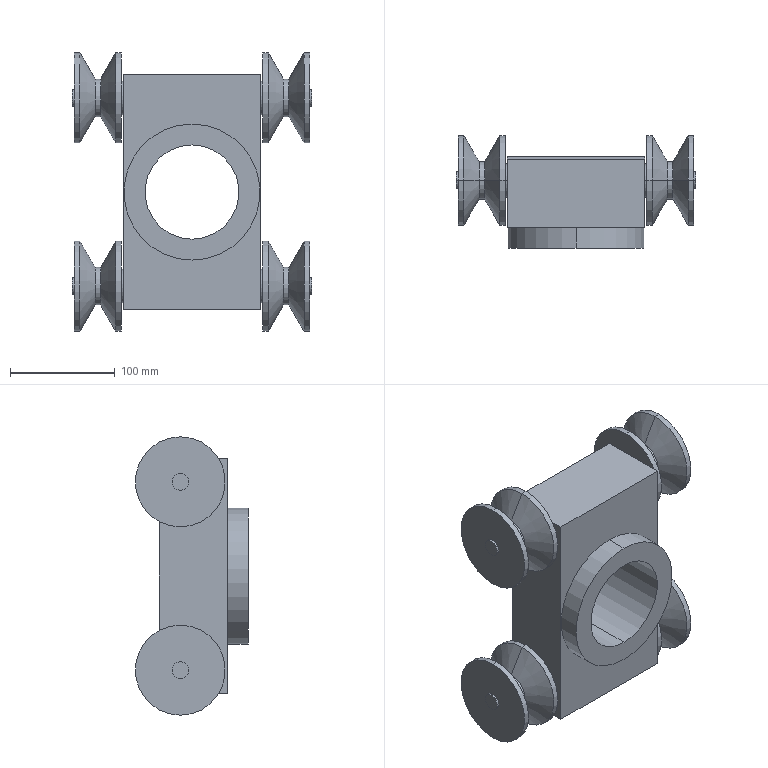Part | SolidWorks | features ICE 6, LPattern 2, MirrorPattern 2, Revolution 1 | 1 solid | 83 faces | box 229 x 108 x 266 mm | volume 2286238 mm3 | cylinder 46 | plane 21 | cone 16 | commonest cylinder face diameters 86 x16 16 x8 32 x8 36 x8 45 x2 90 x2